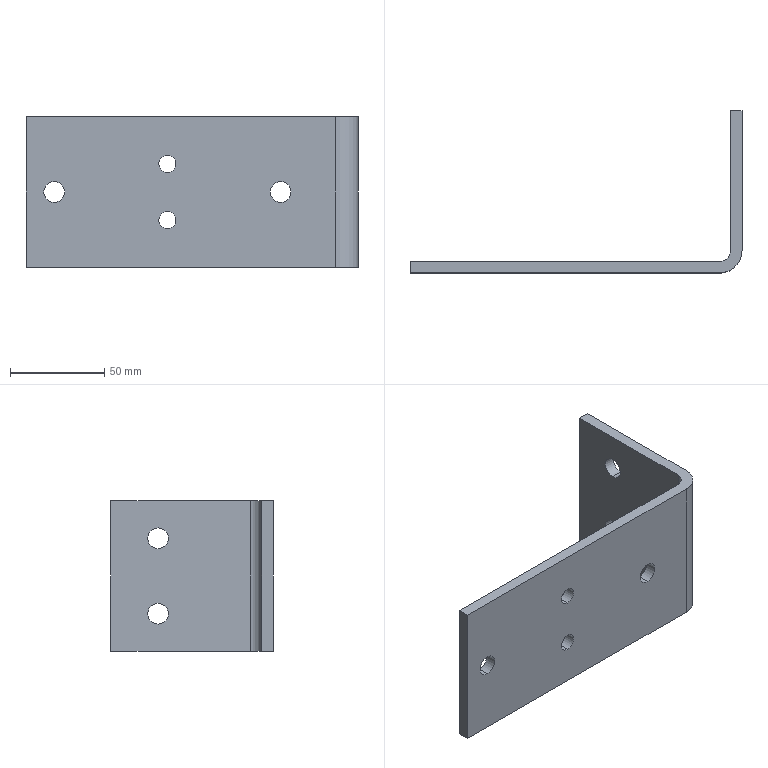Part | SolidWorks | features BaseBody 1 | 1 solid | 22 faces | box 176 x 86 x 80 mm | volume 117965 mm3 | cylinder 14 | plane 8 | commonest cylinder face diameters 11 x8 9.1 x4 12 x1 24 x1
STEP:
#1=CARTESIAN_POINT('',(621.946,-3632.473,1056.971));
#2=VERTEX_POINT('',#1);
#3=CARTESIAN_POINT('',(621.946,-3632.473,1045.971));
#4=VERTEX_POINT('',#3);
#5=CARTESIAN_POINT('',(621.946,-3632.473,1051.471));
#6=DIRECTION('',(0.,-1.,0.));
#7=DIRECTION('',(0.,0.,-1.));
#8=AXIS2_PLACEMENT_3D('',#5,#6,#7);
#9=CIRCLE('',#8,5.5);
#10=EDGE_CURVE('',#2,#4,#9,.T.);
#11=ORIENTED_EDGE('',*,*,#10,.F.);
#12=CARTESIAN_POINT('',(621.946,-3638.473,1056.971));
#13=VERTEX_POINT('',#12);
#14=CARTESIAN_POINT('',(621.946,-3631.032,1056.971));
#15=DIRECTION('',(0.,-1.,0.));
#16=VECTOR('',#15,1000.);
#17=LINE('',#14,#16);
#18=EDGE_CURVE('',#2,#13,#17,.T.);
#19=ORIENTED_EDGE('',*,*,#18,.T.);
#20=CARTESIAN_POINT('',(621.946,-3638.473,1045.971));
#21=VERTEX_POINT('',#20);
#22=CARTESIAN_POINT('',(621.946,-3638.473,1051.471));
#23=DIRECTION('',(0.,1.,0.));
#24=DIRECTION('',(0.,0.,-1.));
#25=AXIS2_PLACEMENT_3D('',#22,#23,#24);
#26=CIRCLE('',#25,5.5);
#27=EDGE_CURVE('',#21,#13,#26,.T.);
#28=ORIENTED_EDGE('',*,*,#27,.F.);
#29=CARTESIAN_POINT('',(621.946,-3631.032,1045.971));
#30=DIRECTION('',(0.,-1.,0.));
#31=VECTOR('',#30,1000.);
#32=LINE('',#29,#31);
#33=EDGE_CURVE('',#4,#21,#32,.T.);
#34=ORIENTED_EDGE('',*,*,#33,.F.);
#35=EDGE_LOOP('',(#11,#19,#28,#34));
#36=FACE_OUTER_BOUND('',#35,.T.);
#37=CARTESIAN_POINT('',(621.946,-3631.032,1051.471));
#38=DIRECTION('',(0.,-1.,0.));
#39=DIRECTION('',(0.,0.,-1.));
#40=AXIS2_PLACEMENT_3D('',#37,#38,#39);
#41=CYLINDRICAL_SURFACE('',#40,5.5);
#42=ADVANCED_FACE('',(#36),#41,.F.);
#43=CARTESIAN_POINT('',(741.946,-3638.473,1045.971));
#44=VERTEX_POINT('',#43);
#45=CARTESIAN_POINT('',(741.946,-3638.473,1056.971));
#46=VERTEX_POINT('',#45);
#47=CARTESIAN_POINT('',(741.946,-3638.473,1051.471));
#48=DIRECTION('',(0.,1.,0.));
#49=DIRECTION('',(0.,0.,1.));
#50=AXIS2_PLACEMENT_3D('',#47,#48,#49);
#51=CIRCLE('',#50,5.5);
#52=EDGE_CURVE('',#44,#46,#51,.T.);
#53=ORIENTED_EDGE('',*,*,#52,.F.);
#54=CARTESIAN_POINT('',(741.946,-3632.473,1045.971));
#55=VERTEX_POINT('',#54);
#56=CARTESIAN_POINT('',(741.946,-3631.032,1045.971));
#57=DIRECTION('',(0.,1.,0.));
#58=VECTOR('',#57,1000.);
#59=LINE('',#56,#58);
#60=EDGE_CURVE('',#44,#55,#59,.T.);
#61=ORIENTED_EDGE('',*,*,#60,.T.);
#62=CARTESIAN_POINT('',(741.946,-3632.473,1056.971));
#63=VERTEX_POINT('',#62);
#64=CARTESIAN_POINT('',(741.946,-3632.473,1051.471));
#65=DIRECTION('',(0.,-1.,0.));
#66=DIRECTION('',(0.,0.,1.));
#67=AXIS2_PLACEMENT_3D('',#64,#65,#66);
#68=CIRCLE('',#67,5.5);
#69=EDGE_CURVE('',#63,#55,#68,.T.);
#70=ORIENTED_EDGE('',*,*,#69,.F.);
#71=CARTESIAN_POINT('',(741.946,-3631.032,1056.971));
#72=DIRECTION('',(0.,1.,0.));
#73=VECTOR('',#72,1000.);
#74=LINE('',#71,#73);
#75=EDGE_CURVE('',#46,#63,#74,.T.);
#76=ORIENTED_EDGE('',*,*,#75,.F.);
#77=EDGE_LOOP('',(#53,#61,#70,#76));
#78=FACE_OUTER_BOUND('',#77,.T.);
#79=CARTESIAN_POINT('',(741.946,-3631.032,1051.471));
#80=DIRECTION('',(0.,1.,0.));
#81=DIRECTION('',(0.,0.,1.));
#82=AXIS2_PLACEMENT_3D('',#79,#80,#81);
#83=CYLINDRICAL_SURFACE('',#82,5.5);
#84=ADVANCED_FACE('',(#78),#83,.F.);
#85=CARTESIAN_POINT('',(681.946,-3632.473,1071.021));
#86=VERTEX_POINT('',#85);
#87=CARTESIAN_POINT('',(681.946,-3632.473,1061.921));
#88=VERTEX_POINT('',#87);
#89=CARTESIAN_POINT('',(681.946,-3632.473,1066.471));
#90=DIRECTION('',(0.,-1.,0.));
#91=DIRECTION('',(0.,0.,-1.));
#92=AXIS2_PLACEMENT_3D('',#89,#90,#91);
#93=CIRCLE('',#92,4.55);
#94=EDGE_CURVE('',#86,#88,#93,.T.);
#95=ORIENTED_EDGE('',*,*,#94,.F.);
#96=CARTESIAN_POINT('',(681.946,-3638.473,1071.021));
#97=VERTEX_POINT('',#96);
#98=CARTESIAN_POINT('',(681.946,-3643.612,1071.021));
#99=DIRECTION('',(0.,-1.,0.));
#100=VECTOR('',#99,1000.);
#101=LINE('',#98,#100);
#102=EDGE_CURVE('',#86,#97,#101,.T.);
#103=ORIENTED_EDGE('',*,*,#102,.T.);
#104=CARTESIAN_POINT('',(681.946,-3638.473,1061.921));
#105=VERTEX_POINT('',#104);
#106=CARTESIAN_POINT('',(681.946,-3638.473,1066.471));
#107=DIRECTION('',(0.,1.,0.));
#108=DIRECTION('',(0.,0.,-1.));
#109=AXIS2_PLACEMENT_3D('',#106,#107,#108);
#110=CIRCLE('',#109,4.55);
#111=EDGE_CURVE('',#105,#97,#110,.T.);
#112=ORIENTED_EDGE('',*,*,#111,.F.);
#113=CARTESIAN_POINT('',(681.946,-3643.612,1061.921));
#114=DIRECTION('',(0.,-1.,0.));
#115=VECTOR('',#114,1000.);
#116=LINE('',#113,#115);
#117=EDGE_CURVE('',#88,#105,#116,.T.);
#118=ORIENTED_EDGE('',*,*,#117,.F.);
#119=EDGE_LOOP('',(#95,#103,#112,#118));
#120=FACE_OUTER_BOUND('',#119,.T.);
#121=CARTESIAN_POINT('',(681.946,-3643.612,1066.471));
#122=DIRECTION('',(0.,-1.,0.));
#123=DIRECTION('',(0.,0.,-1.));
#124=AXIS2_PLACEMENT_3D('',#121,#122,#123);
#125=CYLINDRICAL_SURFACE('',#124,4.55);
#126=ADVANCED_FACE('',(#120),#125,.F.);
#127=CARTESIAN_POINT('',(681.946,-3632.473,1041.021));
#128=VERTEX_POINT('',#127);
#129=CARTESIAN_POINT('',(681.946,-3632.473,1031.921));
#130=VERTEX_POINT('',#129);
#131=CARTESIAN_POINT('',(681.946,-3632.473,1036.471));
#132=DIRECTION('',(0.,-1.,0.));
#133=DIRECTION('',(0.,0.,-1.));
#134=AXIS2_PLACEMENT_3D('',#131,#132,#133);
#135=CIRCLE('',#134,4.55);
#136=EDGE_CURVE('',#128,#130,#135,.T.);
#137=ORIENTED_EDGE('',*,*,#136,.F.);
#138=CARTESIAN_POINT('',(681.946,-3638.473,1041.021));
#139=VERTEX_POINT('',#138);
#140=CARTESIAN_POINT('',(681.946,-3643.612,1041.021));
#141=DIRECTION('',(0.,-1.,0.));
#142=VECTOR('',#141,1000.);
#143=LINE('',#140,#142);
#144=EDGE_CURVE('',#128,#139,#143,.T.);
#145=ORIENTED_EDGE('',*,*,#144,.T.);
#146=CARTESIAN_POINT('',(681.946,-3638.473,1031.921));
#147=VERTEX_POINT('',#146);
#148=CARTESIAN_POINT('',(681.946,-3638.473,1036.471));
#149=DIRECTION('',(0.,1.,0.));
#150=DIRECTION('',(0.,0.,-1.));
#151=AXIS2_PLACEMENT_3D('',#148,#149,#150);
#152=CIRCLE('',#151,4.55);
#153=EDGE_CURVE('',#147,#139,#152,.T.);
#154=ORIENTED_EDGE('',*,*,#153,.F.);
#155=CARTESIAN_POINT('',(681.946,-3643.612,1031.921));
#156=DIRECTION('',(0.,-1.,0.));
#157=VECTOR('',#156,1000.);
#158=LINE('',#155,#157);
#159=EDGE_CURVE('',#130,#147,#158,.T.);
#160=ORIENTED_EDGE('',*,*,#159,.F.);
#161=EDGE_LOOP('',(#137,#145,#154,#160));
#162=FACE_OUTER_BOUND('',#161,.T.);
#163=CARTESIAN_POINT('',(681.946,-3643.612,1036.471));
#164=DIRECTION('',(0.,-1.,0.));
#165=DIRECTION('',(0.,0.,-1.));
#166=AXIS2_PLACEMENT_3D('',#163,#164,#165);
#167=CYLINDRICAL_SURFACE('',#166,4.55);
#168=ADVANCED_FACE('',(#162),#167,.F.);
#169=CARTESIAN_POINT('',(782.946,-3577.473,1065.971));
#170=VERTEX_POINT('',#169);
#171=CARTESIAN_POINT('',(782.946,-3577.473,1076.971));
#172=VERTEX_POINT('',#171);
#173=CARTESIAN_POINT('',(782.946,-3577.473,1071.471));
#174=DIRECTION('',(-1.,0.,0.));
#175=DIRECTION('',(0.,0.,1.));
#176=AXIS2_PLACEMENT_3D('',#173,#174,#175);
#177=CIRCLE('',#176,5.5);
#178=EDGE_CURVE('',#170,#172,#177,.T.);
#179=ORIENTED_EDGE('',*,*,#178,.F.);
#180=CARTESIAN_POINT('',(776.946,-3577.473,1065.971));
#181=VERTEX_POINT('',#180);
#182=CARTESIAN_POINT('',(762.945,-3577.473,1065.971));
#183=DIRECTION('',(-1.,0.,0.));
#184=VECTOR('',#183,1000.);
#185=LINE('',#182,#184);
#186=EDGE_CURVE('',#170,#181,#185,.T.);
#187=ORIENTED_EDGE('',*,*,#186,.T.);
#188=CARTESIAN_POINT('',(776.946,-3577.473,1076.971));
#189=VERTEX_POINT('',#188);
#190=CARTESIAN_POINT('',(776.946,-3577.473,1071.471));
#191=DIRECTION('',(1.,0.,0.));
#192=DIRECTION('',(0.,0.,1.));
#193=AXIS2_PLACEMENT_3D('',#190,#191,#192);
#194=CIRCLE('',#193,5.5);
#195=EDGE_CURVE('',#189,#181,#194,.T.);
#196=ORIENTED_EDGE('',*,*,#195,.F.);
#197=CARTESIAN_POINT('',(762.945,-3577.473,1076.971));
#198=DIRECTION('',(-1.,0.,0.));
#199=VECTOR('',#198,1000.);
#200=LINE('',#197,#199);
#201=EDGE_CURVE('',#172,#189,#200,.T.);
#202=ORIENTED_EDGE('',*,*,#201,.F.);
#203=EDGE_LOOP('',(#179,#187,#196,#202));
#204=FACE_OUTER_BOUND('',#203,.T.);
#205=CARTESIAN_POINT('',(762.945,-3577.473,1071.471));
#206=DIRECTION('',(-1.,0.,0.));
#207=DIRECTION('',(0.,0.,1.));
#208=AXIS2_PLACEMENT_3D('',#205,#206,#207);
#209=CYLINDRICAL_SURFACE('',#208,5.5);
#210=ADVANCED_FACE('',(#204),#209,.F.);
#211=CARTESIAN_POINT('',(782.946,-3577.473,1025.971));
#212=VERTEX_POINT('',#211);
#213=CARTESIAN_POINT('',(782.946,-3577.473,1036.971));
#214=VERTEX_POINT('',#213);
#215=CARTESIAN_POINT('',(782.946,-3577.473,1031.471));
#216=DIRECTION('',(-1.,0.,0.));
#217=DIRECTION('',(0.,0.,1.));
#218=AXIS2_PLACEMENT_3D('',#215,#216,#217);
#219=CIRCLE('',#218,5.5);
#220=EDGE_CURVE('',#212,#214,#219,.T.);
#221=ORIENTED_EDGE('',*,*,#220,.F.);
#222=CARTESIAN_POINT('',(776.946,-3577.473,1025.971));
#223=VERTEX_POINT('',#222);
#224=CARTESIAN_POINT('',(762.945,-3577.473,1025.971));
#225=DIRECTION('',(-1.,0.,0.));
#226=VECTOR('',#225,1000.);
#227=LINE('',#224,#226);
#228=EDGE_CURVE('',#212,#223,#227,.T.);
#229=ORIENTED_EDGE('',*,*,#228,.T.);
#230=CARTESIAN_POINT('',(776.946,-3577.473,1036.971));
#231=VERTEX_POINT('',#230);
#232=CARTESIAN_POINT('',(776.946,-3577.473,1031.471));
#233=DIRECTION('',(1.,0.,0.));
#234=DIRECTION('',(0.,0.,1.));
#235=AXIS2_PLACEMENT_3D('',#232,#233,#234);
#236=CIRCLE('',#235,5.5);
#237=EDGE_CURVE('',#231,#223,#236,.T.);
#238=ORIENTED_EDGE('',*,*,#237,.F.);
#239=CARTESIAN_POINT('',(762.945,-3577.473,1036.971));
#240=DIRECTION('',(-1.,0.,0.));
#241=VECTOR('',#240,1000.);
#242=LINE('',#239,#241);
#243=EDGE_CURVE('',#214,#231,#242,.T.);
#244=ORIENTED_EDGE('',*,*,#243,.F.);
#245=EDGE_LOOP('',(#221,#229,#238,#244));
#246=FACE_OUTER_BOUND('',#245,.T.);
#247=CARTESIAN_POINT('',(762.945,-3577.473,1031.471));
#248=DIRECTION('',(-1.,0.,0.));
#249=DIRECTION('',(0.,0.,1.));
#250=AXIS2_PLACEMENT_3D('',#247,#248,#249);
#251=CYLINDRICAL_SURFACE('',#250,5.5);
#252=ADVANCED_FACE('',(#246),#251,.F.);
#253=CARTESIAN_POINT('',(770.946,-3632.473,1011.471));
#254=VERTEX_POINT('',#253);
#255=CARTESIAN_POINT('',(606.946,-3632.473,1011.471));
#256=VERTEX_POINT('',#255);
#257=CARTESIAN_POINT('',(656.946,-3632.473,1011.471));
#258=DIRECTION('',(-1.,0.,0.));
#259=VECTOR('',#258,1000.);
#260=LINE('',#257,#259);
#261=EDGE_CURVE('',#254,#256,#260,.T.);
#262=ORIENTED_EDGE('',*,*,#261,.T.);
#263=CARTESIAN_POINT('',(606.946,-3632.473,1091.471));
#264=VERTEX_POINT('',#263);
#265=CARTESIAN_POINT('',(606.946,-3632.473,1011.471));
#266=DIRECTION('',(0.,0.,1.));
#267=VECTOR('',#266,1000.);
#268=LINE('',#265,#267);
#269=EDGE_CURVE('',#256,#264,#268,.T.);
#270=ORIENTED_EDGE('',*,*,#269,.T.);
#271=CARTESIAN_POINT('',(770.946,-3632.473,1091.471));
#272=VERTEX_POINT('',#271);
#273=CARTESIAN_POINT('',(656.946,-3632.473,1091.471));
#274=DIRECTION('',(1.,0.,0.));
#275=VECTOR('',#274,1000.);
#276=LINE('',#273,#275);
#277=EDGE_CURVE('',#264,#272,#276,.T.);
#278=ORIENTED_EDGE('',*,*,#277,.T.);
#279=CARTESIAN_POINT('',(770.946,-3632.473,1011.471));
#280=DIRECTION('',(0.,0.,-1.));
#281=VECTOR('',#280,1000.);
#282=LINE('',#279,#281);
#283=EDGE_CURVE('',#272,#254,#282,.T.);
#284=ORIENTED_EDGE('',*,*,#283,.T.);
#285=EDGE_LOOP('',(#262,#270,#278,#284));
#286=FACE_OUTER_BOUND('',#285,.T.);
#287=CARTESIAN_POINT('',(621.946,-3632.473,1051.471));
#288=DIRECTION('',(0.,-1.,0.));
#289=DIRECTION('',(0.,0.,-1.));
#290=AXIS2_PLACEMENT_3D('',#287,#288,#289);
#291=CIRCLE('',#290,5.5);
#292=EDGE_CURVE('',#4,#2,#291,.T.);
#293=ORIENTED_EDGE('',*,*,#292,.T.);
#294=ORIENTED_EDGE('',*,*,#10,.T.);
#295=EDGE_LOOP('',(#293,#294));
#296=FACE_BOUND('',#295,.T.);
#297=ORIENTED_EDGE('',*,*,#69,.T.);
#298=CARTESIAN_POINT('',(741.946,-3632.473,1051.471));
#299=DIRECTION('',(0.,-1.,0.));
#300=DIRECTION('',(0.,0.,1.));
#301=AXIS2_PLACEMENT_3D('',#298,#299,#300);
#302=CIRCLE('',#301,5.5);
#303=EDGE_CURVE('',#55,#63,#302,.T.);
#304=ORIENTED_EDGE('',*,*,#303,.T.);
#305=EDGE_LOOP('',(#297,#304));
#306=FACE_BOUND('',#305,.T.);
#307=CARTESIAN_POINT('',(681.946,-3632.473,1066.471));
#308=DIRECTION('',(0.,-1.,0.));
#309=DIRECTION('',(0.,0.,-1.));
#310=AXIS2_PLACEMENT_3D('',#307,#308,#309);
#311=CIRCLE('',#310,4.55);
#312=EDGE_CURVE('',#88,#86,#311,.T.);
#313=ORIENTED_EDGE('',*,*,#312,.T.);
#314=ORIENTED_EDGE('',*,*,#94,.T.);
#315=EDGE_LOOP('',(#313,#314));
#316=FACE_BOUND('',#315,.T.);
#317=CARTESIAN_POINT('',(681.946,-3632.473,1036.471));
#318=DIRECTION('',(0.,-1.,0.));
#319=DIRECTION('',(0.,0.,-1.));
#320=AXIS2_PLACEMENT_3D('',#317,#318,#319);
#321=CIRCLE('',#320,4.55);
#322=EDGE_CURVE('',#130,#128,#321,.T.);
#323=ORIENTED_EDGE('',*,*,#322,.T.);
#324=ORIENTED_EDGE('',*,*,#136,.T.);
#325=EDGE_LOOP('',(#323,#324));
#326=FACE_BOUND('',#325,.T.);
#327=CARTESIAN_POINT('',(656.946,-3632.473,1011.471));
#328=DIRECTION('',(0.,1.,0.));
#329=DIRECTION('',(0.,0.,1.));
#330=AXIS2_PLACEMENT_3D('',#327,#328,#329);
#331=PLANE('',#330);
#332=ADVANCED_FACE('',(#286,#296,#306,#316,#326),#331,.T.);
#333=CARTESIAN_POINT('',(606.946,-3638.473,1011.471));
#334=VERTEX_POINT('',#333);
#335=CARTESIAN_POINT('',(606.946,-3638.473,1011.471));
#336=DIRECTION('',(0.,-1.,0.));
#337=VECTOR('',#336,1000.);
#338=LINE('',#335,#337);
#339=EDGE_CURVE('',#256,#334,#338,.T.);
#340=ORIENTED_EDGE('',*,*,#339,.T.);
#341=CARTESIAN_POINT('',(606.946,-3638.473,1091.471));
#342=VERTEX_POINT('',#341);
#343=CARTESIAN_POINT('',(606.946,-3638.473,1011.471));
#344=DIRECTION('',(0.,0.,1.));
#345=VECTOR('',#344,1000.);
#346=LINE('',#343,#345);
#347=EDGE_CURVE('',#334,#342,#346,.T.);
#348=ORIENTED_EDGE('',*,*,#347,.T.);
#349=CARTESIAN_POINT('',(606.946,-3638.473,1091.471));
#350=DIRECTION('',(0.,1.,0.));
#351=VECTOR('',#350,1000.);
#352=LINE('',#349,#351);
#353=EDGE_CURVE('',#342,#264,#352,.T.);
#354=ORIENTED_EDGE('',*,*,#353,.T.);
#355=ORIENTED_EDGE('',*,*,#269,.F.);
#356=EDGE_LOOP('',(#340,#348,#354,#355));
#357=FACE_OUTER_BOUND('',#356,.T.);
#358=CARTESIAN_POINT('',(606.946,-3638.473,1011.471));
#359=DIRECTION('',(-1.,0.,0.));
#360=DIRECTION('',(0.,0.,1.));
#361=AXIS2_PLACEMENT_3D('',#358,#359,#360);
#362=PLANE('',#361);
#363=ADVANCED_FACE('',(#357),#362,.T.);
#364=CARTESIAN_POINT('',(770.946,-3638.473,1011.471));
#365=VERTEX_POINT('',#364);
#366=CARTESIAN_POINT('',(741.835,-3638.473,1011.471));
#367=DIRECTION('',(1.,0.,0.));
#368=VECTOR('',#367,1000.);
#369=LINE('',#366,#368);
#370=EDGE_CURVE('',#334,#365,#369,.T.);
#371=ORIENTED_EDGE('',*,*,#370,.F.);
#372=ORIENTED_EDGE('',*,*,#339,.F.);
#373=ORIENTED_EDGE('',*,*,#261,.F.);
#374=CARTESIAN_POINT('',(776.946,-3626.473,1011.471));
#375=VERTEX_POINT('',#374);
#376=CARTESIAN_POINT('',(770.946,-3626.473,1011.471));
#377=DIRECTION('',(0.,0.,-1.));
#378=DIRECTION('',(1.,0.,0.));
#379=AXIS2_PLACEMENT_3D('',#376,#377,#378);
#380=CIRCLE('',#379,6.);
#381=EDGE_CURVE('',#375,#254,#380,.T.);
#382=ORIENTED_EDGE('',*,*,#381,.F.);
#383=CARTESIAN_POINT('',(776.946,-3552.473,1011.471));
#384=VERTEX_POINT('',#383);
#385=CARTESIAN_POINT('',(776.946,-3617.734,1011.471));
#386=DIRECTION('',(0.,-1.,0.));
#387=VECTOR('',#386,1000.);
#388=LINE('',#385,#387);
#389=EDGE_CURVE('',#384,#375,#388,.T.);
#390=ORIENTED_EDGE('',*,*,#389,.F.);
#391=CARTESIAN_POINT('',(782.946,-3552.473,1011.471));
#392=VERTEX_POINT('',#391);
#393=CARTESIAN_POINT('',(741.835,-3552.473,1011.471));
#394=DIRECTION('',(-1.,0.,0.));
#395=VECTOR('',#394,1000.);
#396=LINE('',#393,#395);
#397=EDGE_CURVE('',#392,#384,#396,.T.);
#398=ORIENTED_EDGE('',*,*,#397,.F.);
#399=CARTESIAN_POINT('',(782.946,-3626.473,1011.471));
#400=VERTEX_POINT('',#399);
#401=CARTESIAN_POINT('',(782.946,-3617.734,1011.471));
#402=DIRECTION('',(0.,1.,0.));
#403=VECTOR('',#402,1000.);
#404=LINE('',#401,#403);
#405=EDGE_CURVE('',#400,#392,#404,.T.);
#406=ORIENTED_EDGE('',*,*,#405,.F.);
#407=CARTESIAN_POINT('',(770.946,-3626.473,1011.471));
#408=DIRECTION('',(0.,0.,1.));
#409=DIRECTION('',(1.,0.,0.));
#410=AXIS2_PLACEMENT_3D('',#407,#408,#409);
#411=CIRCLE('',#410,12.);
#412=EDGE_CURVE('',#365,#400,#411,.T.);
#413=ORIENTED_EDGE('',*,*,#412,.F.);
#414=EDGE_LOOP('',(#371,#372,#373,#382,#390,#398,#406,#413));
#415=FACE_OUTER_BOUND('',#414,.T.);
#416=CARTESIAN_POINT('',(741.835,-3617.734,1011.471));
#417=DIRECTION('',(0.,0.,1.));
#418=DIRECTION('',(1.,0.,0.));
#419=AXIS2_PLACEMENT_3D('',#416,#417,#418);
#420=PLANE('',#419);
#421=ADVANCED_FACE('',(#415),#420,.F.);
#422=ORIENTED_EDGE('',*,*,#381,.T.);
#423=ORIENTED_EDGE('',*,*,#283,.F.);
#424=CARTESIAN_POINT('',(776.946,-3626.473,1091.471));
#425=VERTEX_POINT('',#424);
#426=CARTESIAN_POINT('',(770.946,-3626.473,1091.471));
#427=DIRECTION('',(0.,0.,1.));
#428=DIRECTION('',(1.,0.,0.));
#429=AXIS2_PLACEMENT_3D('',#426,#427,#428);
#430=CIRCLE('',#429,6.);
#431=EDGE_CURVE('',#272,#425,#430,.T.);
#432=ORIENTED_EDGE('',*,*,#431,.T.);
#433=CARTESIAN_POINT('',(776.946,-3626.473,1011.471));
#434=DIRECTION('',(0.,0.,-1.));
#435=VECTOR('',#434,1000.);
#436=LINE('',#433,#435);
#437=EDGE_CURVE('',#425,#375,#436,.T.);
#438=ORIENTED_EDGE('',*,*,#437,.T.);
#439=EDGE_LOOP('',(#422,#423,#432,#438));
#440=FACE_OUTER_BOUND('',#439,.T.);
#441=CARTESIAN_POINT('',(770.946,-3626.473,1011.471));
#442=DIRECTION('',(0.,0.,1.));
#443=DIRECTION('',(1.,0.,0.));
#444=AXIS2_PLACEMENT_3D('',#441,#442,#443);
#445=CYLINDRICAL_SURFACE('',#444,6.);
#446=ADVANCED_FACE('',(#440),#445,.F.);
#447=ORIENTED_EDGE('',*,*,#277,.F.);
#448=ORIENTED_EDGE('',*,*,#353,.F.);
#449=CARTESIAN_POINT('',(770.946,-3638.473,1091.471));
#450=VERTEX_POINT('',#449);
#451=CARTESIAN_POINT('',(741.835,-3638.473,1091.471));
#452=DIRECTION('',(1.,0.,0.));
#453=VECTOR('',#452,1000.);
#454=LINE('',#451,#453);
#455=EDGE_CURVE('',#342,#450,#454,.T.);
#456=ORIENTED_EDGE('',*,*,#455,.T.);
#457=CARTESIAN_POINT('',(782.946,-3626.473,1091.471));
#458=VERTEX_POINT('',#457);
#459=CARTESIAN_POINT('',(770.946,-3626.473,1091.471));
#460=DIRECTION('',(0.,0.,1.));
#461=DIRECTION('',(1.,0.,0.));
#462=AXIS2_PLACEMENT_3D('',#459,#460,#461);
#463=CIRCLE('',#462,12.);
#464=EDGE_CURVE('',#450,#458,#463,.T.);
#465=ORIENTED_EDGE('',*,*,#464,.T.);
#466=CARTESIAN_POINT('',(782.946,-3552.473,1091.471));
#467=VERTEX_POINT('',#466);
#468=CARTESIAN_POINT('',(782.946,-3617.734,1091.471));
#469=DIRECTION('',(0.,1.,0.));
#470=VECTOR('',#469,1000.);
#471=LINE('',#468,#470);
#472=EDGE_CURVE('',#458,#467,#471,.T.);
#473=ORIENTED_EDGE('',*,*,#472,.T.);
#474=CARTESIAN_POINT('',(776.946,-3552.473,1091.471));
#475=VERTEX_POINT('',#474);
#476=CARTESIAN_POINT('',(741.835,-3552.473,1091.471));
#477=DIRECTION('',(-1.,0.,0.));
#478=VECTOR('',#477,1000.);
#479=LINE('',#476,#478);
#480=EDGE_CURVE('',#467,#475,#479,.T.);
#481=ORIENTED_EDGE('',*,*,#480,.T.);
#482=CARTESIAN_POINT('',(776.946,-3617.734,1091.471));
#483=DIRECTION('',(0.,-1.,0.));
#484=VECTOR('',#483,1000.);
#485=LINE('',#482,#484);
#486=EDGE_CURVE('',#475,#425,#485,.T.);
#487=ORIENTED_EDGE('',*,*,#486,.T.);
#488=ORIENTED_EDGE('',*,*,#431,.F.);
#489=EDGE_LOOP('',(#447,#448,#456,#465,#473,#481,#487,#488));
#490=FACE_OUTER_BOUND('',#489,.T.);
#491=CARTESIAN_POINT('',(741.835,-3617.734,1091.471));
#492=DIRECTION('',(0.,0.,1.));
#493=DIRECTION('',(1.,0.,0.));
#494=AXIS2_PLACEMENT_3D('',#491,#492,#493);
#495=PLANE('',#494);
#496=ADVANCED_FACE('',(#490),#495,.T.);
#497=ORIENTED_EDGE('',*,*,#18,.F.);
#498=ORIENTED_EDGE('',*,*,#292,.F.);
#499=ORIENTED_EDGE('',*,*,#33,.T.);
#500=CARTESIAN_POINT('',(621.946,-3638.473,1051.471));
#501=DIRECTION('',(0.,1.,0.));
#502=DIRECTION('',(0.,0.,-1.));
#503=AXIS2_PLACEMENT_3D('',#500,#501,#502);
#504=CIRCLE('',#503,5.5);
#505=EDGE_CURVE('',#13,#21,#504,.T.);
#506=ORIENTED_EDGE('',*,*,#505,.F.);
#507=EDGE_LOOP('',(#497,#498,#499,#506));
#508=FACE_OUTER_BOUND('',#507,.T.);
#509=CARTESIAN_POINT('',(621.946,-3631.032,1051.471));
#510=DIRECTION('',(0.,-1.,0.));
#511=DIRECTION('',(0.,0.,-1.));
#512=AXIS2_PLACEMENT_3D('',#509,#510,#511);
#513=CYLINDRICAL_SURFACE('',#512,5.5);
#514=ADVANCED_FACE('',(#508),#513,.F.);
#515=ORIENTED_EDGE('',*,*,#60,.F.);
#516=CARTESIAN_POINT('',(741.946,-3638.473,1051.471));
#517=DIRECTION('',(0.,1.,0.));
#518=DIRECTION('',(0.,0.,1.));
#519=AXIS2_PLACEMENT_3D('',#516,#517,#518);
#520=CIRCLE('',#519,5.5);
#521=EDGE_CURVE('',#46,#44,#520,.T.);
#522=ORIENTED_EDGE('',*,*,#521,.F.);
#523=ORIENTED_EDGE('',*,*,#75,.T.);
#524=ORIENTED_EDGE('',*,*,#303,.F.);
#525=EDGE_LOOP('',(#515,#522,#523,#524));
#526=FACE_OUTER_BOUND('',#525,.T.);
#527=CARTESIAN_POINT('',(741.946,-3631.032,1051.471));
#528=DIRECTION('',(0.,1.,0.));
#529=DIRECTION('',(0.,0.,1.));
#530=AXIS2_PLACEMENT_3D('',#527,#528,#529);
#531=CYLINDRICAL_SURFACE('',#530,5.5);
#532=ADVANCED_FACE('',(#526),#531,.F.);
#533=ORIENTED_EDGE('',*,*,#102,.F.);
#534=ORIENTED_EDGE('',*,*,#312,.F.);
#535=ORIENTED_EDGE('',*,*,#117,.T.);
#536=CARTESIAN_POINT('',(681.946,-3638.473,1066.471));
#537=DIRECTION('',(0.,1.,0.));
#538=DIRECTION('',(0.,0.,-1.));
#539=AXIS2_PLACEMENT_3D('',#536,#537,#538);
#540=CIRCLE('',#539,4.55);
#541=EDGE_CURVE('',#97,#105,#540,.T.);
#542=ORIENTED_EDGE('',*,*,#541,.F.);
#543=EDGE_LOOP('',(#533,#534,#535,#542));
#544=FACE_OUTER_BOUND('',#543,.T.);
#545=CARTESIAN_POINT('',(681.946,-3643.612,1066.471));
#546=DIRECTION('',(0.,-1.,0.));
#547=DIRECTION('',(0.,0.,-1.));
#548=AXIS2_PLACEMENT_3D('',#545,#546,#547);
#549=CYLINDRICAL_SURFACE('',#548,4.55);
#550=ADVANCED_FACE('',(#544),#549,.F.);
#551=ORIENTED_EDGE('',*,*,#144,.F.);
#552=ORIENTED_EDGE('',*,*,#322,.F.);
#553=ORIENTED_EDGE('',*,*,#159,.T.);
#554=CARTESIAN_POINT('',(681.946,-3638.473,1036.471));
#555=DIRECTION('',(0.,1.,0.));
#556=DIRECTION('',(0.,0.,-1.));
#557=AXIS2_PLACEMENT_3D('',#554,#555,#556);
#558=CIRCLE('',#557,4.55);
#559=EDGE_CURVE('',#139,#147,#558,.T.);
#560=ORIENTED_EDGE('',*,*,#559,.F.);
#561=EDGE_LOOP('',(#551,#552,#553,#560));
#562=FACE_OUTER_BOUND('',#561,.T.);
#563=CARTESIAN_POINT('',(681.946,-3643.612,1036.471));
#564=DIRECTION('',(0.,-1.,0.));
#565=DIRECTION('',(0.,0.,-1.));
#566=AXIS2_PLACEMENT_3D('',#563,#564,#565);
#567=CYLINDRICAL_SURFACE('',#566,4.55);
#568=ADVANCED_FACE('',(#562),#567,.F.);
#569=ORIENTED_EDGE('',*,*,#370,.T.);
#570=CARTESIAN_POINT('',(770.946,-3638.473,1011.471));
#571=DIRECTION('',(0.,0.,1.));
#572=VECTOR('',#571,1000.);
#573=LINE('',#570,#572);
#574=EDGE_CURVE('',#365,#450,#573,.T.);
#575=ORIENTED_EDGE('',*,*,#574,.T.);
#576=ORIENTED_EDGE('',*,*,#455,.F.);
#577=ORIENTED_EDGE('',*,*,#347,.F.);
#578=EDGE_LOOP('',(#569,#575,#576,#577));
#579=FACE_OUTER_BOUND('',#578,.T.);
#580=ORIENTED_EDGE('',*,*,#27,.T.);
#581=ORIENTED_EDGE('',*,*,#505,.T.);
#582=EDGE_LOOP('',(#580,#581));
#583=FACE_BOUND('',#582,.T.);
#584=ORIENTED_EDGE('',*,*,#521,.T.);
#585=ORIENTED_EDGE('',*,*,#52,.T.);
#586=EDGE_LOOP('',(#584,#585));
#587=FACE_BOUND('',#586,.T.);
#588=ORIENTED_EDGE('',*,*,#111,.T.);
#589=ORIENTED_EDGE('',*,*,#541,.T.);
#590=EDGE_LOOP('',(#588,#589));
#591=FACE_BOUND('',#590,.T.);
#592=ORIENTED_EDGE('',*,*,#153,.T.);
#593=ORIENTED_EDGE('',*,*,#559,.T.);
#594=EDGE_LOOP('',(#592,#593));
#595=FACE_BOUND('',#594,.T.);
#596=CARTESIAN_POINT('',(770.946,-3638.473,1011.471));
#597=DIRECTION('',(0.,-1.,0.));
#598=DIRECTION('',(1.,0.,0.));
#599=AXIS2_PLACEMENT_3D('',#596,#597,#598);
#600=PLANE('',#599);
#601=ADVANCED_FACE('',(#579,#583,#587,#591,#595),#600,.T.);
#602=ORIENTED_EDGE('',*,*,#412,.T.);
#603=CARTESIAN_POINT('',(782.946,-3626.473,1011.471));
#604=DIRECTION('',(0.,0.,1.));
#605=VECTOR('',#604,1000.);
#606=LINE('',#603,#605);
#607=EDGE_CURVE('',#400,#458,#606,.T.);
#608=ORIENTED_EDGE('',*,*,#607,.T.);
#609=ORIENTED_EDGE('',*,*,#464,.F.);
#610=ORIENTED_EDGE('',*,*,#574,.F.);
#611=EDGE_LOOP('',(#602,#608,#609,#610));
#612=FACE_OUTER_BOUND('',#611,.T.);
#613=CARTESIAN_POINT('',(770.946,-3626.473,1011.471));
#614=DIRECTION('',(0.,0.,1.));
#615=DIRECTION('',(1.,0.,0.));
#616=AXIS2_PLACEMENT_3D('',#613,#614,#615);
#617=CYLINDRICAL_SURFACE('',#616,12.);
#618=ADVANCED_FACE('',(#612),#617,.T.);
#619=ORIENTED_EDGE('',*,*,#389,.T.);
#620=ORIENTED_EDGE('',*,*,#437,.F.);
#621=ORIENTED_EDGE('',*,*,#486,.F.);
#622=CARTESIAN_POINT('',(776.946,-3552.473,1011.471));
#623=DIRECTION('',(0.,0.,-1.));
#624=VECTOR('',#623,1000.);
#625=LINE('',#622,#624);
#626=EDGE_CURVE('',#475,#384,#625,.T.);
#627=ORIENTED_EDGE('',*,*,#626,.T.);
#628=EDGE_LOOP('',(#619,#620,#621,#627));
#629=FACE_OUTER_BOUND('',#628,.T.);
#630=ORIENTED_EDGE('',*,*,#195,.T.);
#631=CARTESIAN_POINT('',(776.946,-3577.473,1071.471));
#632=DIRECTION('',(1.,0.,0.));
#633=DIRECTION('',(0.,0.,1.));
#634=AXIS2_PLACEMENT_3D('',#631,#632,#633);
#635=CIRCLE('',#634,5.5);
#636=EDGE_CURVE('',#181,#189,#635,.T.);
#637=ORIENTED_EDGE('',*,*,#636,.T.);
#638=EDGE_LOOP('',(#630,#637));
#639=FACE_BOUND('',#638,.T.);
#640=ORIENTED_EDGE('',*,*,#237,.T.);
#641=CARTESIAN_POINT('',(776.946,-3577.473,1031.471));
#642=DIRECTION('',(1.,0.,0.));
#643=DIRECTION('',(0.,0.,1.));
#644=AXIS2_PLACEMENT_3D('',#641,#642,#643);
#645=CIRCLE('',#644,5.5);
#646=EDGE_CURVE('',#223,#231,#645,.T.);
#647=ORIENTED_EDGE('',*,*,#646,.T.);
#648=EDGE_LOOP('',(#640,#647));
#649=FACE_BOUND('',#648,.T.);
#650=CARTESIAN_POINT('',(776.946,-3626.473,1011.471));
#651=DIRECTION('',(-1.,0.,0.));
#652=DIRECTION('',(0.,0.,1.));
#653=AXIS2_PLACEMENT_3D('',#650,#651,#652);
#654=PLANE('',#653);
#655=ADVANCED_FACE('',(#629,#639,#649),#654,.T.);
#656=ORIENTED_EDGE('',*,*,#397,.T.);
#657=ORIENTED_EDGE('',*,*,#626,.F.);
#658=ORIENTED_EDGE('',*,*,#480,.F.);
#659=CARTESIAN_POINT('',(782.946,-3552.473,1011.471));
#660=DIRECTION('',(0.,0.,-1.));
#661=VECTOR('',#660,1000.);
#662=LINE('',#659,#661);
#663=EDGE_CURVE('',#467,#392,#662,.T.);
#664=ORIENTED_EDGE('',*,*,#663,.T.);
#665=EDGE_LOOP('',(#656,#657,#658,#664));
#666=FACE_OUTER_BOUND('',#665,.T.);
#667=CARTESIAN_POINT('',(776.946,-3552.473,1011.471));
#668=DIRECTION('',(0.,1.,0.));
#669=DIRECTION('',(0.,0.,1.));
#670=AXIS2_PLACEMENT_3D('',#667,#668,#669);
#671=PLANE('',#670);
#672=ADVANCED_FACE('',(#666),#671,.T.);
#673=ORIENTED_EDGE('',*,*,#405,.T.);
#674=ORIENTED_EDGE('',*,*,#663,.F.);
#675=ORIENTED_EDGE('',*,*,#472,.F.);
#676=ORIENTED_EDGE('',*,*,#607,.F.);
#677=EDGE_LOOP('',(#673,#674,#675,#676));
#678=FACE_OUTER_BOUND('',#677,.T.);
#679=CARTESIAN_POINT('',(782.946,-3577.473,1071.471));
#680=DIRECTION('',(-1.,0.,0.));
#681=DIRECTION('',(0.,0.,1.));
#682=AXIS2_PLACEMENT_3D('',#679,#680,#681);
#683=CIRCLE('',#682,5.5);
#684=EDGE_CURVE('',#172,#170,#683,.T.);
#685=ORIENTED_EDGE('',*,*,#684,.T.);
#686=ORIENTED_EDGE('',*,*,#178,.T.);
#687=EDGE_LOOP('',(#685,#686));
#688=FACE_BOUND('',#687,.T.);
#689=CARTESIAN_POINT('',(782.946,-3577.473,1031.471));
#690=DIRECTION('',(-1.,0.,0.));
#691=DIRECTION('',(0.,0.,1.));
#692=AXIS2_PLACEMENT_3D('',#689,#690,#691);
#693=CIRCLE('',#692,5.5);
#694=EDGE_CURVE('',#214,#212,#693,.T.);
#695=ORIENTED_EDGE('',*,*,#694,.T.);
#696=ORIENTED_EDGE('',*,*,#220,.T.);
#697=EDGE_LOOP('',(#695,#696));
#698=FACE_BOUND('',#697,.T.);
#699=CARTESIAN_POINT('',(782.946,-3552.473,1011.471));
#700=DIRECTION('',(1.,0.,0.));
#701=DIRECTION('',(0.,0.,-1.));
#702=AXIS2_PLACEMENT_3D('',#699,#700,#701);
#703=PLANE('',#702);
#704=ADVANCED_FACE('',(#678,#688,#698),#703,.T.);
#705=ORIENTED_EDGE('',*,*,#186,.F.);
#706=ORIENTED_EDGE('',*,*,#684,.F.);
#707=ORIENTED_EDGE('',*,*,#201,.T.);
#708=ORIENTED_EDGE('',*,*,#636,.F.);
#709=EDGE_LOOP('',(#705,#706,#707,#708));
#710=FACE_OUTER_BOUND('',#709,.T.);
#711=CARTESIAN_POINT('',(762.945,-3577.473,1071.471));
#712=DIRECTION('',(-1.,0.,0.));
#713=DIRECTION('',(0.,0.,1.));
#714=AXIS2_PLACEMENT_3D('',#711,#712,#713);
#715=CYLINDRICAL_SURFACE('',#714,5.5);
#716=ADVANCED_FACE('',(#710),#715,.F.);
#717=ORIENTED_EDGE('',*,*,#228,.F.);
#718=ORIENTED_EDGE('',*,*,#694,.F.);
#719=ORIENTED_EDGE('',*,*,#243,.T.);
#720=ORIENTED_EDGE('',*,*,#646,.F.);
#721=EDGE_LOOP('',(#717,#718,#719,#720));
#722=FACE_OUTER_BOUND('',#721,.T.);
#723=CARTESIAN_POINT('',(762.945,-3577.473,1031.471));
#724=DIRECTION('',(-1.,0.,0.));
#725=DIRECTION('',(0.,0.,1.));
#726=AXIS2_PLACEMENT_3D('',#723,#724,#725);
#727=CYLINDRICAL_SURFACE('',#726,5.5);
#728=ADVANCED_FACE('',(#722),#727,.F.);
#729=CLOSED_SHELL('',(#42,#84,#126,#168,#210,#252,#332,#363,#421,#446,#496,#514,#532,#550,#568,#601,#618,#655,#672,#704,#716,#728));
#730=MANIFOLD_SOLID_BREP('',#729);
#731=CARTESIAN_POINT('',(0.,0.,0.));
#732=DIRECTION('',(0.,0.,1.));
#733=DIRECTION('',(1.,0.,0.));
#734=AXIS2_PLACEMENT_3D('',#731,#732,#733);
#735=(LENGTH_UNIT()NAMED_UNIT(*)SI_UNIT(.MILLI.,.METRE.));
#736=UNCERTAINTY_MEASURE_WITH_UNIT(LENGTH_MEASURE(0.00001),#735,'','');
#737=(NAMED_UNIT(*)PLANE_ANGLE_UNIT()SI_UNIT($,.RADIAN.));
#738=(NAMED_UNIT(*)SI_UNIT($,.STERADIAN.)SOLID_ANGLE_UNIT());
#739=(GEOMETRIC_REPRESENTATION_CONTEXT(3)GLOBAL_UNCERTAINTY_ASSIGNED_CONTEXT((#736))GLOBAL_UNIT_ASSIGNED_CONTEXT((#735,#737,#738))REPRESENTATION_CONTEXT('',''));
#740=ADVANCED_BREP_SHAPE_REPRESENTATION('',(#730,#734),#739);